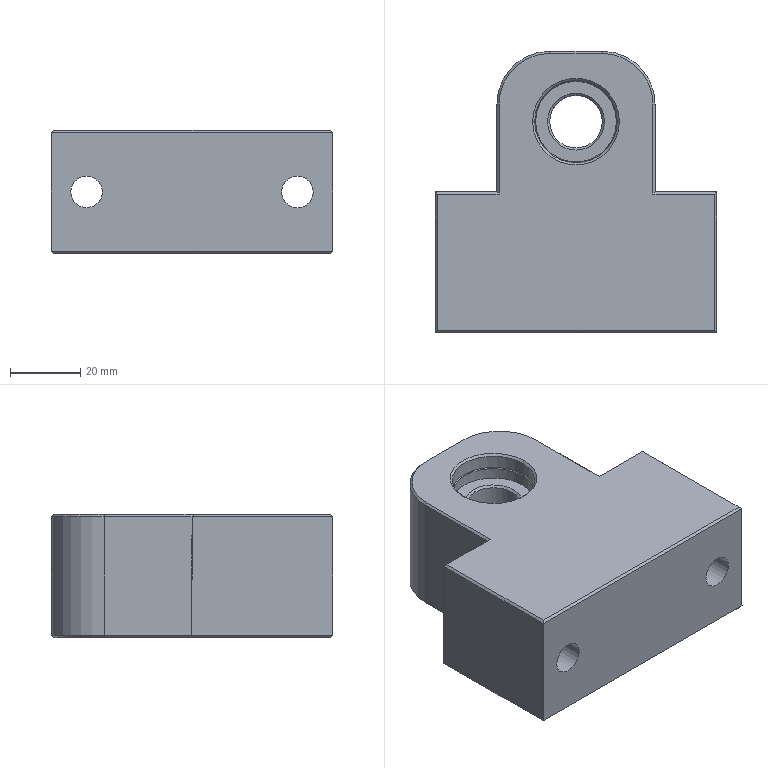Part | SolidWorks | features BaseBody 1 | 1 solid | 67 faces | box 80 x 80 x 35 mm | volume 146595 mm3 | plane 31 | cylinder 20 | cone 16 | commonest cylinder face diameters 9 x4 13.5 x4 23 x4 30 x4 15 x2 23.5 x2